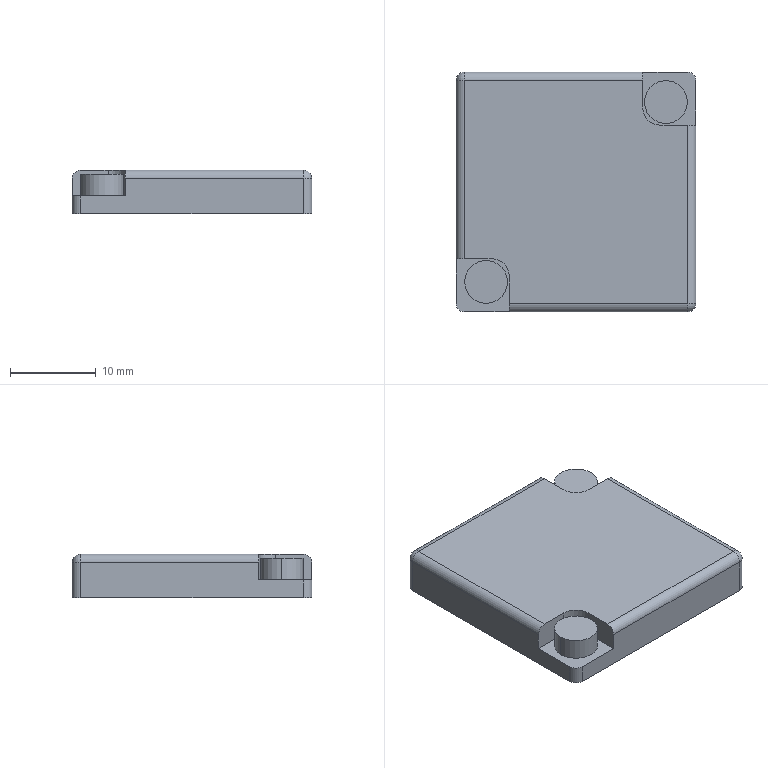Part | STEP file | AW30-03E_AW3020A Gauge_30 | 1 solid | 30 faces | box 28 x 28 x 5.1 mm | volume 3850 mm3 | cylinder 14 | plane 14 | sphere 2 | commonest cylinder face diameters 2 x8 5 x4 4 x2
STEP:
#1=CARTESIAN_POINT('',(-8.,-10.5,-0.5));
#2=VERTEX_POINT('',#1);
#3=CARTESIAN_POINT('',(-13.,-10.5,-0.5));
#4=VERTEX_POINT('',#3);
#5=CARTESIAN_POINT('',(-10.5,-10.5,-0.5));
#6=DIRECTION('',(0.,0.,1.));
#7=DIRECTION('',(-1.,0.,0.));
#8=AXIS2_PLACEMENT_3D('',#5,#6,#7);
#9=CIRCLE('',#8,2.5);
#10=EDGE_CURVE('',#2,#4,#9,.T.);
#11=ORIENTED_EDGE('',*,*,#10,.F.);
#12=CARTESIAN_POINT('',(-8.,-10.5,-3.));
#13=VERTEX_POINT('',#12);
#14=CARTESIAN_POINT('',(-8.,-10.5,-0.5));
#15=DIRECTION('',(0.,0.,-1.));
#16=VECTOR('',#15,1000.);
#17=LINE('',#14,#16);
#18=EDGE_CURVE('',#2,#13,#17,.T.);
#19=ORIENTED_EDGE('',*,*,#18,.T.);
#20=CARTESIAN_POINT('',(-13.,-10.5,-3.));
#21=VERTEX_POINT('',#20);
#22=CARTESIAN_POINT('',(-10.5,-10.5,-3.));
#23=DIRECTION('',(0.,0.,1.));
#24=DIRECTION('',(-1.,0.,0.));
#25=AXIS2_PLACEMENT_3D('',#22,#23,#24);
#26=CIRCLE('',#25,2.5);
#27=EDGE_CURVE('',#13,#21,#26,.T.);
#28=ORIENTED_EDGE('',*,*,#27,.T.);
#29=CARTESIAN_POINT('',(-13.,-10.5,-0.5));
#30=DIRECTION('',(0.,0.,-1.));
#31=VECTOR('',#30,1000.);
#32=LINE('',#29,#31);
#33=EDGE_CURVE('',#4,#21,#32,.T.);
#34=ORIENTED_EDGE('',*,*,#33,.F.);
#35=EDGE_LOOP('',(#11,#19,#28,#34));
#36=FACE_OUTER_BOUND('',#35,.T.);
#37=CARTESIAN_POINT('',(-10.5,-10.5,-0.5));
#38=DIRECTION('',(0.,0.,-1.));
#39=DIRECTION('',(-1.,0.,0.));
#40=AXIS2_PLACEMENT_3D('',#37,#38,#39);
#41=CYLINDRICAL_SURFACE('',#40,2.5);
#42=ADVANCED_FACE('',(#36),#41,.T.);
#43=CARTESIAN_POINT('',(13.,10.5,-0.5));
#44=VERTEX_POINT('',#43);
#45=CARTESIAN_POINT('',(8.,10.5,-0.5));
#46=VERTEX_POINT('',#45);
#47=CARTESIAN_POINT('',(10.5,10.5,-0.5));
#48=DIRECTION('',(0.,0.,1.));
#49=DIRECTION('',(1.,0.,0.));
#50=AXIS2_PLACEMENT_3D('',#47,#48,#49);
#51=CIRCLE('',#50,2.5);
#52=EDGE_CURVE('',#44,#46,#51,.T.);
#53=ORIENTED_EDGE('',*,*,#52,.F.);
#54=CARTESIAN_POINT('',(13.,10.5,-3.));
#55=VERTEX_POINT('',#54);
#56=CARTESIAN_POINT('',(13.,10.5,-0.5));
#57=DIRECTION('',(0.,0.,-1.));
#58=VECTOR('',#57,1000.);
#59=LINE('',#56,#58);
#60=EDGE_CURVE('',#44,#55,#59,.T.);
#61=ORIENTED_EDGE('',*,*,#60,.T.);
#62=CARTESIAN_POINT('',(8.,10.5,-3.));
#63=VERTEX_POINT('',#62);
#64=CARTESIAN_POINT('',(10.5,10.5,-3.));
#65=DIRECTION('',(0.,0.,1.));
#66=DIRECTION('',(1.,0.,0.));
#67=AXIS2_PLACEMENT_3D('',#64,#65,#66);
#68=CIRCLE('',#67,2.5);
#69=EDGE_CURVE('',#55,#63,#68,.T.);
#70=ORIENTED_EDGE('',*,*,#69,.T.);
#71=CARTESIAN_POINT('',(8.,10.5,-0.5));
#72=DIRECTION('',(0.,0.,-1.));
#73=VECTOR('',#72,1000.);
#74=LINE('',#71,#73);
#75=EDGE_CURVE('',#46,#63,#74,.T.);
#76=ORIENTED_EDGE('',*,*,#75,.F.);
#77=EDGE_LOOP('',(#53,#61,#70,#76));
#78=FACE_OUTER_BOUND('',#77,.T.);
#79=CARTESIAN_POINT('',(10.5,10.5,-0.5));
#80=DIRECTION('',(0.,0.,-1.));
#81=DIRECTION('',(-1.,0.,0.));
#82=AXIS2_PLACEMENT_3D('',#79,#80,#81);
#83=CYLINDRICAL_SURFACE('',#82,2.5);
#84=ADVANCED_FACE('',(#78),#83,.T.);
#85=CARTESIAN_POINT('',(-13.,-14.,-3.));
#86=VERTEX_POINT('',#85);
#87=CARTESIAN_POINT('',(-7.8,-14.,-3.));
#88=VERTEX_POINT('',#87);
#89=CARTESIAN_POINT('',(-14.,-14.,-3.));
#90=DIRECTION('',(1.,0.,0.));
#91=VECTOR('',#90,1000.);
#92=LINE('',#89,#91);
#93=EDGE_CURVE('',#86,#88,#92,.T.);
#94=ORIENTED_EDGE('',*,*,#93,.T.);
#95=CARTESIAN_POINT('',(-7.8,-9.8,-3.));
#96=VERTEX_POINT('',#95);
#97=CARTESIAN_POINT('',(-7.8,-14.,-3.));
#98=DIRECTION('',(0.,1.,0.));
#99=VECTOR('',#98,1000.);
#100=LINE('',#97,#99);
#101=EDGE_CURVE('',#88,#96,#100,.T.);
#102=ORIENTED_EDGE('',*,*,#101,.T.);
#103=CARTESIAN_POINT('',(-9.8,-7.8,-3.));
#104=VERTEX_POINT('',#103);
#105=CARTESIAN_POINT('',(-9.8,-9.8,-3.));
#106=DIRECTION('',(0.,0.,1.));
#107=DIRECTION('',(-1.,0.,0.));
#108=AXIS2_PLACEMENT_3D('',#105,#106,#107);
#109=CIRCLE('',#108,2.);
#110=EDGE_CURVE('',#96,#104,#109,.T.);
#111=ORIENTED_EDGE('',*,*,#110,.T.);
#112=CARTESIAN_POINT('',(-14.,-7.8,-3.));
#113=VERTEX_POINT('',#112);
#114=CARTESIAN_POINT('',(-14.,-7.8,-3.));
#115=DIRECTION('',(-1.,0.,0.));
#116=VECTOR('',#115,1000.);
#117=LINE('',#114,#116);
#118=EDGE_CURVE('',#104,#113,#117,.T.);
#119=ORIENTED_EDGE('',*,*,#118,.T.);
#120=CARTESIAN_POINT('',(-14.,-13.,-3.));
#121=VERTEX_POINT('',#120);
#122=CARTESIAN_POINT('',(-14.,-14.,-3.));
#123=DIRECTION('',(0.,-1.,0.));
#124=VECTOR('',#123,1000.);
#125=LINE('',#122,#124);
#126=EDGE_CURVE('',#113,#121,#125,.T.);
#127=ORIENTED_EDGE('',*,*,#126,.T.);
#128=CARTESIAN_POINT('',(-13.,-13.,-3.));
#129=DIRECTION('',(0.,0.,-1.));
#130=DIRECTION('',(1.,0.,0.));
#131=AXIS2_PLACEMENT_3D('',#128,#129,#130);
#132=CIRCLE('',#131,1.);
#133=EDGE_CURVE('',#86,#121,#132,.T.);
#134=ORIENTED_EDGE('',*,*,#133,.F.);
#135=EDGE_LOOP('',(#94,#102,#111,#119,#127,#134));
#136=FACE_OUTER_BOUND('',#135,.T.);
#137=CARTESIAN_POINT('',(-10.5,-10.5,-3.));
#138=DIRECTION('',(0.,0.,1.));
#139=DIRECTION('',(-1.,0.,0.));
#140=AXIS2_PLACEMENT_3D('',#137,#138,#139);
#141=CIRCLE('',#140,2.5);
#142=EDGE_CURVE('',#21,#13,#141,.T.);
#143=ORIENTED_EDGE('',*,*,#142,.F.);
#144=ORIENTED_EDGE('',*,*,#27,.F.);
#145=EDGE_LOOP('',(#143,#144));
#146=FACE_BOUND('',#145,.T.);
#147=CARTESIAN_POINT('',(-9.8,-9.8,-3.));
#148=DIRECTION('',(0.,0.,1.));
#149=DIRECTION('',(-1.,0.,0.));
#150=AXIS2_PLACEMENT_3D('',#147,#148,#149);
#151=PLANE('',#150);
#152=ADVANCED_FACE('',(#136,#146),#151,.T.);
#153=CARTESIAN_POINT('',(-13.,-14.,-5.1));
#154=VERTEX_POINT('',#153);
#155=CARTESIAN_POINT('',(-13.,-14.,-5.1));
#156=DIRECTION('',(0.,0.,-1.));
#157=VECTOR('',#156,1000.);
#158=LINE('',#155,#157);
#159=EDGE_CURVE('',#86,#154,#158,.T.);
#160=ORIENTED_EDGE('',*,*,#159,.F.);
#161=ORIENTED_EDGE('',*,*,#133,.T.);
#162=CARTESIAN_POINT('',(-14.,-13.,-5.1));
#163=VERTEX_POINT('',#162);
#164=CARTESIAN_POINT('',(-14.,-13.,-5.1));
#165=DIRECTION('',(0.,0.,1.));
#166=VECTOR('',#165,1000.);
#167=LINE('',#164,#166);
#168=EDGE_CURVE('',#163,#121,#167,.T.);
#169=ORIENTED_EDGE('',*,*,#168,.F.);
#170=CARTESIAN_POINT('',(-13.,-13.,-5.1));
#171=DIRECTION('',(0.,0.,-1.));
#172=DIRECTION('',(-1.,0.,0.));
#173=AXIS2_PLACEMENT_3D('',#170,#171,#172);
#174=CIRCLE('',#173,1.);
#175=EDGE_CURVE('',#154,#163,#174,.T.);
#176=ORIENTED_EDGE('',*,*,#175,.F.);
#177=EDGE_LOOP('',(#160,#161,#169,#176));
#178=FACE_OUTER_BOUND('',#177,.T.);
#179=CARTESIAN_POINT('',(-13.,-13.,-5.1));
#180=DIRECTION('',(0.,0.,1.));
#181=DIRECTION('',(1.,0.,0.));
#182=AXIS2_PLACEMENT_3D('',#179,#180,#181);
#183=CYLINDRICAL_SURFACE('',#182,1.);
#184=ADVANCED_FACE('',(#178),#183,.T.);
#185=CARTESIAN_POINT('',(13.,14.,-3.));
#186=VERTEX_POINT('',#185);
#187=CARTESIAN_POINT('',(7.8,14.,-3.));
#188=VERTEX_POINT('',#187);
#189=CARTESIAN_POINT('',(14.,14.,-3.));
#190=DIRECTION('',(-1.,0.,0.));
#191=VECTOR('',#190,1000.);
#192=LINE('',#189,#191);
#193=EDGE_CURVE('',#186,#188,#192,.T.);
#194=ORIENTED_EDGE('',*,*,#193,.T.);
#195=CARTESIAN_POINT('',(7.8,9.8,-3.));
#196=VERTEX_POINT('',#195);
#197=CARTESIAN_POINT('',(7.8,14.,-3.));
#198=DIRECTION('',(0.,-1.,0.));
#199=VECTOR('',#198,1000.);
#200=LINE('',#197,#199);
#201=EDGE_CURVE('',#188,#196,#200,.T.);
#202=ORIENTED_EDGE('',*,*,#201,.T.);
#203=CARTESIAN_POINT('',(9.8,7.8,-3.));
#204=VERTEX_POINT('',#203);
#205=CARTESIAN_POINT('',(9.8,9.8,-3.));
#206=DIRECTION('',(0.,0.,1.));
#207=DIRECTION('',(1.,0.,0.));
#208=AXIS2_PLACEMENT_3D('',#205,#206,#207);
#209=CIRCLE('',#208,2.);
#210=EDGE_CURVE('',#196,#204,#209,.T.);
#211=ORIENTED_EDGE('',*,*,#210,.T.);
#212=CARTESIAN_POINT('',(14.,7.8,-3.));
#213=VERTEX_POINT('',#212);
#214=CARTESIAN_POINT('',(14.,7.8,-3.));
#215=DIRECTION('',(1.,0.,0.));
#216=VECTOR('',#215,1000.);
#217=LINE('',#214,#216);
#218=EDGE_CURVE('',#204,#213,#217,.T.);
#219=ORIENTED_EDGE('',*,*,#218,.T.);
#220=CARTESIAN_POINT('',(14.,13.,-3.));
#221=VERTEX_POINT('',#220);
#222=CARTESIAN_POINT('',(14.,14.,-3.));
#223=DIRECTION('',(0.,1.,0.));
#224=VECTOR('',#223,1000.);
#225=LINE('',#222,#224);
#226=EDGE_CURVE('',#213,#221,#225,.T.);
#227=ORIENTED_EDGE('',*,*,#226,.T.);
#228=CARTESIAN_POINT('',(13.,13.,-3.));
#229=DIRECTION('',(0.,0.,-1.));
#230=DIRECTION('',(1.,0.,0.));
#231=AXIS2_PLACEMENT_3D('',#228,#229,#230);
#232=CIRCLE('',#231,1.);
#233=EDGE_CURVE('',#186,#221,#232,.T.);
#234=ORIENTED_EDGE('',*,*,#233,.F.);
#235=EDGE_LOOP('',(#194,#202,#211,#219,#227,#234));
#236=FACE_OUTER_BOUND('',#235,.T.);
#237=CARTESIAN_POINT('',(10.5,10.5,-3.));
#238=DIRECTION('',(0.,0.,1.));
#239=DIRECTION('',(1.,0.,0.));
#240=AXIS2_PLACEMENT_3D('',#237,#238,#239);
#241=CIRCLE('',#240,2.5);
#242=EDGE_CURVE('',#63,#55,#241,.T.);
#243=ORIENTED_EDGE('',*,*,#242,.F.);
#244=ORIENTED_EDGE('',*,*,#69,.F.);
#245=EDGE_LOOP('',(#243,#244));
#246=FACE_BOUND('',#245,.T.);
#247=CARTESIAN_POINT('',(9.8,9.8,-3.));
#248=DIRECTION('',(0.,0.,1.));
#249=DIRECTION('',(1.,0.,0.));
#250=AXIS2_PLACEMENT_3D('',#247,#248,#249);
#251=PLANE('',#250);
#252=ADVANCED_FACE('',(#236,#246),#251,.T.);
#253=CARTESIAN_POINT('',(13.,14.,-5.1));
#254=VERTEX_POINT('',#253);
#255=CARTESIAN_POINT('',(13.,14.,-5.1));
#256=DIRECTION('',(0.,0.,-1.));
#257=VECTOR('',#256,1000.);
#258=LINE('',#255,#257);
#259=EDGE_CURVE('',#186,#254,#258,.T.);
#260=ORIENTED_EDGE('',*,*,#259,.F.);
#261=ORIENTED_EDGE('',*,*,#233,.T.);
#262=CARTESIAN_POINT('',(14.,13.,-5.1));
#263=VERTEX_POINT('',#262);
#264=CARTESIAN_POINT('',(14.,13.,-5.1));
#265=DIRECTION('',(0.,0.,1.));
#266=VECTOR('',#265,1000.);
#267=LINE('',#264,#266);
#268=EDGE_CURVE('',#263,#221,#267,.T.);
#269=ORIENTED_EDGE('',*,*,#268,.F.);
#270=CARTESIAN_POINT('',(13.,13.,-5.1));
#271=DIRECTION('',(0.,0.,-1.));
#272=DIRECTION('',(-1.,0.,0.));
#273=AXIS2_PLACEMENT_3D('',#270,#271,#272);
#274=CIRCLE('',#273,1.);
#275=EDGE_CURVE('',#254,#263,#274,.T.);
#276=ORIENTED_EDGE('',*,*,#275,.F.);
#277=EDGE_LOOP('',(#260,#261,#269,#276));
#278=FACE_OUTER_BOUND('',#277,.T.);
#279=CARTESIAN_POINT('',(13.,13.,-5.1));
#280=DIRECTION('',(0.,0.,1.));
#281=DIRECTION('',(1.,0.,0.));
#282=AXIS2_PLACEMENT_3D('',#279,#280,#281);
#283=CYLINDRICAL_SURFACE('',#282,1.);
#284=ADVANCED_FACE('',(#278),#283,.T.);
#285=CARTESIAN_POINT('',(14.,7.8,-1.));
#286=VERTEX_POINT('',#285);
#287=CARTESIAN_POINT('',(14.,7.8,-3.));
#288=DIRECTION('',(0.,0.,1.));
#289=VECTOR('',#288,1000.);
#290=LINE('',#287,#289);
#291=EDGE_CURVE('',#213,#286,#290,.T.);
#292=ORIENTED_EDGE('',*,*,#291,.T.);
#293=CARTESIAN_POINT('',(14.,-13.,-1.));
#294=VERTEX_POINT('',#293);
#295=CARTESIAN_POINT('',(14.,-14.,-1.));
#296=DIRECTION('',(0.,-1.,0.));
#297=VECTOR('',#296,1000.);
#298=LINE('',#295,#297);
#299=EDGE_CURVE('',#286,#294,#298,.T.);
#300=ORIENTED_EDGE('',*,*,#299,.T.);
#301=CARTESIAN_POINT('',(14.,-13.,-5.1));
#302=VERTEX_POINT('',#301);
#303=CARTESIAN_POINT('',(14.,-13.,-5.1));
#304=DIRECTION('',(0.,0.,-1.));
#305=VECTOR('',#304,1000.);
#306=LINE('',#303,#305);
#307=EDGE_CURVE('',#294,#302,#306,.T.);
#308=ORIENTED_EDGE('',*,*,#307,.T.);
#309=CARTESIAN_POINT('',(14.,14.,-5.1));
#310=DIRECTION('',(0.,1.,0.));
#311=VECTOR('',#310,1000.);
#312=LINE('',#309,#311);
#313=EDGE_CURVE('',#302,#263,#312,.T.);
#314=ORIENTED_EDGE('',*,*,#313,.T.);
#315=ORIENTED_EDGE('',*,*,#268,.T.);
#316=ORIENTED_EDGE('',*,*,#226,.F.);
#317=EDGE_LOOP('',(#292,#300,#308,#314,#315,#316));
#318=FACE_OUTER_BOUND('',#317,.T.);
#319=CARTESIAN_POINT('',(14.,14.,-5.1));
#320=DIRECTION('',(1.,0.,0.));
#321=DIRECTION('',(0.,1.,0.));
#322=AXIS2_PLACEMENT_3D('',#319,#320,#321);
#323=PLANE('',#322);
#324=ADVANCED_FACE('',(#318),#323,.T.);
#325=CARTESIAN_POINT('',(-7.8,-14.,-1.));
#326=VERTEX_POINT('',#325);
#327=CARTESIAN_POINT('',(-7.8,-14.,-3.));
#328=DIRECTION('',(0.,0.,1.));
#329=VECTOR('',#328,1000.);
#330=LINE('',#327,#329);
#331=EDGE_CURVE('',#88,#326,#330,.T.);
#332=ORIENTED_EDGE('',*,*,#331,.F.);
#333=ORIENTED_EDGE('',*,*,#93,.F.);
#334=ORIENTED_EDGE('',*,*,#159,.T.);
#335=CARTESIAN_POINT('',(13.,-14.,-5.1));
#336=VERTEX_POINT('',#335);
#337=CARTESIAN_POINT('',(14.,-14.,-5.1));
#338=DIRECTION('',(1.,0.,0.));
#339=VECTOR('',#338,1000.);
#340=LINE('',#337,#339);
#341=EDGE_CURVE('',#154,#336,#340,.T.);
#342=ORIENTED_EDGE('',*,*,#341,.T.);
#343=CARTESIAN_POINT('',(13.,-14.,-1.));
#344=VERTEX_POINT('',#343);
#345=CARTESIAN_POINT('',(13.,-14.,-5.1));
#346=DIRECTION('',(0.,0.,1.));
#347=VECTOR('',#346,1000.);
#348=LINE('',#345,#347);
#349=EDGE_CURVE('',#336,#344,#348,.T.);
#350=ORIENTED_EDGE('',*,*,#349,.T.);
#351=CARTESIAN_POINT('',(-14.,-14.,-1.));
#352=DIRECTION('',(-1.,0.,0.));
#353=VECTOR('',#352,1000.);
#354=LINE('',#351,#353);
#355=EDGE_CURVE('',#344,#326,#354,.T.);
#356=ORIENTED_EDGE('',*,*,#355,.T.);
#357=EDGE_LOOP('',(#332,#333,#334,#342,#350,#356));
#358=FACE_OUTER_BOUND('',#357,.T.);
#359=CARTESIAN_POINT('',(14.,-14.,-5.1));
#360=DIRECTION('',(0.,-1.,0.));
#361=DIRECTION('',(1.,0.,0.));
#362=AXIS2_PLACEMENT_3D('',#359,#360,#361);
#363=PLANE('',#362);
#364=ADVANCED_FACE('',(#358),#363,.T.);
#365=CARTESIAN_POINT('',(-14.,-7.8,-1.));
#366=VERTEX_POINT('',#365);
#367=CARTESIAN_POINT('',(-14.,-7.8,-3.));
#368=DIRECTION('',(0.,0.,1.));
#369=VECTOR('',#368,1000.);
#370=LINE('',#367,#369);
#371=EDGE_CURVE('',#113,#366,#370,.T.);
#372=ORIENTED_EDGE('',*,*,#371,.T.);
#373=CARTESIAN_POINT('',(-14.,13.,-1.));
#374=VERTEX_POINT('',#373);
#375=CARTESIAN_POINT('',(-14.,14.,-1.));
#376=DIRECTION('',(0.,1.,0.));
#377=VECTOR('',#376,1000.);
#378=LINE('',#375,#377);
#379=EDGE_CURVE('',#366,#374,#378,.T.);
#380=ORIENTED_EDGE('',*,*,#379,.T.);
#381=CARTESIAN_POINT('',(-14.,13.,-5.1));
#382=VERTEX_POINT('',#381);
#383=CARTESIAN_POINT('',(-14.,13.,-5.1));
#384=DIRECTION('',(0.,0.,-1.));
#385=VECTOR('',#384,1000.);
#386=LINE('',#383,#385);
#387=EDGE_CURVE('',#374,#382,#386,.T.);
#388=ORIENTED_EDGE('',*,*,#387,.T.);
#389=CARTESIAN_POINT('',(-14.,14.,-5.1));
#390=DIRECTION('',(0.,-1.,0.));
#391=VECTOR('',#390,1000.);
#392=LINE('',#389,#391);
#393=EDGE_CURVE('',#382,#163,#392,.T.);
#394=ORIENTED_EDGE('',*,*,#393,.T.);
#395=ORIENTED_EDGE('',*,*,#168,.T.);
#396=ORIENTED_EDGE('',*,*,#126,.F.);
#397=EDGE_LOOP('',(#372,#380,#388,#394,#395,#396));
#398=FACE_OUTER_BOUND('',#397,.T.);
#399=CARTESIAN_POINT('',(-14.,14.,-5.1));
#400=DIRECTION('',(-1.,0.,0.));
#401=DIRECTION('',(0.,-1.,0.));
#402=AXIS2_PLACEMENT_3D('',#399,#400,#401);
#403=PLANE('',#402);
#404=ADVANCED_FACE('',(#398),#403,.T.);
#405=CARTESIAN_POINT('',(7.8,14.,-1.));
#406=VERTEX_POINT('',#405);
#407=CARTESIAN_POINT('',(7.8,14.,-3.));
#408=DIRECTION('',(0.,0.,1.));
#409=VECTOR('',#408,1000.);
#410=LINE('',#407,#409);
#411=EDGE_CURVE('',#188,#406,#410,.T.);
#412=ORIENTED_EDGE('',*,*,#411,.F.);
#413=ORIENTED_EDGE('',*,*,#193,.F.);
#414=ORIENTED_EDGE('',*,*,#259,.T.);
#415=CARTESIAN_POINT('',(-13.,14.,-5.1));
#416=VERTEX_POINT('',#415);
#417=CARTESIAN_POINT('',(14.,14.,-5.1));
#418=DIRECTION('',(-1.,0.,0.));
#419=VECTOR('',#418,1000.);
#420=LINE('',#417,#419);
#421=EDGE_CURVE('',#254,#416,#420,.T.);
#422=ORIENTED_EDGE('',*,*,#421,.T.);
#423=CARTESIAN_POINT('',(-13.,14.,-1.));
#424=VERTEX_POINT('',#423);
#425=CARTESIAN_POINT('',(-13.,14.,-5.1));
#426=DIRECTION('',(0.,0.,1.));
#427=VECTOR('',#426,1000.);
#428=LINE('',#425,#427);
#429=EDGE_CURVE('',#416,#424,#428,.T.);
#430=ORIENTED_EDGE('',*,*,#429,.T.);
#431=CARTESIAN_POINT('',(14.,14.,-1.));
#432=DIRECTION('',(1.,0.,0.));
#433=VECTOR('',#432,1000.);
#434=LINE('',#431,#433);
#435=EDGE_CURVE('',#424,#406,#434,.T.);
#436=ORIENTED_EDGE('',*,*,#435,.T.);
#437=EDGE_LOOP('',(#412,#413,#414,#422,#430,#436));
#438=FACE_OUTER_BOUND('',#437,.T.);
#439=CARTESIAN_POINT('',(14.,14.,-5.1));
#440=DIRECTION('',(0.,1.,0.));
#441=DIRECTION('',(-1.,0.,0.));
#442=AXIS2_PLACEMENT_3D('',#439,#440,#441);
#443=PLANE('',#442);
#444=ADVANCED_FACE('',(#438),#443,.T.);
#445=ORIENTED_EDGE('',*,*,#421,.F.);
#446=ORIENTED_EDGE('',*,*,#275,.T.);
#447=ORIENTED_EDGE('',*,*,#313,.F.);
#448=CARTESIAN_POINT('',(13.,-13.,-5.1));
#449=DIRECTION('',(0.,0.,-1.));
#450=DIRECTION('',(-1.,0.,0.));
#451=AXIS2_PLACEMENT_3D('',#448,#449,#450);
#452=CIRCLE('',#451,1.);
#453=EDGE_CURVE('',#302,#336,#452,.T.);
#454=ORIENTED_EDGE('',*,*,#453,.T.);
#455=ORIENTED_EDGE('',*,*,#341,.F.);
#456=ORIENTED_EDGE('',*,*,#175,.T.);
#457=ORIENTED_EDGE('',*,*,#393,.F.);
#458=CARTESIAN_POINT('',(-13.,13.,-5.1));
#459=DIRECTION('',(0.,0.,-1.));
#460=DIRECTION('',(-1.,0.,0.));
#461=AXIS2_PLACEMENT_3D('',#458,#459,#460);
#462=CIRCLE('',#461,1.);
#463=EDGE_CURVE('',#382,#416,#462,.T.);
#464=ORIENTED_EDGE('',*,*,#463,.T.);
#465=EDGE_LOOP('',(#445,#446,#447,#454,#455,#456,#457,#464));
#466=FACE_OUTER_BOUND('',#465,.T.);
#467=CARTESIAN_POINT('',(14.,-14.,-5.1));
#468=DIRECTION('',(0.,0.,-1.));
#469=DIRECTION('',(-1.,0.,0.));
#470=AXIS2_PLACEMENT_3D('',#467,#468,#469);
#471=PLANE('',#470);
#472=ADVANCED_FACE('',(#466),#471,.T.);
#473=CARTESIAN_POINT('',(-13.,13.,0.));
#474=VERTEX_POINT('',#473);
#475=CARTESIAN_POINT('',(-13.,-7.8,0.));
#476=VERTEX_POINT('',#475);
#477=CARTESIAN_POINT('',(-13.,-14.,0.));
#478=DIRECTION('',(0.,-1.,0.));
#479=VECTOR('',#478,1000.);
#480=LINE('',#477,#479);
#481=EDGE_CURVE('',#474,#476,#480,.T.);
#482=ORIENTED_EDGE('',*,*,#481,.T.);
#483=CARTESIAN_POINT('',(-9.8,-7.8,0.));
#484=VERTEX_POINT('',#483);
#485=CARTESIAN_POINT('',(-14.,-7.8,0.));
#486=DIRECTION('',(-1.,0.,0.));
#487=VECTOR('',#486,1000.);
#488=LINE('',#485,#487);
#489=EDGE_CURVE('',#484,#476,#488,.T.);
#490=ORIENTED_EDGE('',*,*,#489,.F.);
#491=CARTESIAN_POINT('',(-7.8,-9.8,0.));
#492=VERTEX_POINT('',#491);
#493=CARTESIAN_POINT('',(-9.8,-9.8,0.));
#494=DIRECTION('',(0.,0.,1.));
#495=DIRECTION('',(-1.,0.,0.));
#496=AXIS2_PLACEMENT_3D('',#493,#494,#495);
#497=CIRCLE('',#496,2.);
#498=EDGE_CURVE('',#492,#484,#497,.T.);
#499=ORIENTED_EDGE('',*,*,#498,.F.);
#500=CARTESIAN_POINT('',(-7.8,-13.,0.));
#501=VERTEX_POINT('',#500);
#502=CARTESIAN_POINT('',(-7.8,-14.,0.));
#503=DIRECTION('',(0.,1.,0.));
#504=VECTOR('',#503,1000.);
#505=LINE('',#502,#504);
#506=EDGE_CURVE('',#501,#492,#505,.T.);
#507=ORIENTED_EDGE('',*,*,#506,.F.);
#508=CARTESIAN_POINT('',(13.,-13.,0.));
#509=VERTEX_POINT('',#508);
#510=CARTESIAN_POINT('',(14.,-13.,0.));
#511=DIRECTION('',(1.,0.,0.));
#512=VECTOR('',#511,1000.);
#513=LINE('',#510,#512);
#514=EDGE_CURVE('',#501,#509,#513,.T.);
#515=ORIENTED_EDGE('',*,*,#514,.T.);
#516=CARTESIAN_POINT('',(13.,7.8,0.));
#517=VERTEX_POINT('',#516);
#518=CARTESIAN_POINT('',(13.,14.,0.));
#519=DIRECTION('',(0.,1.,0.));
#520=VECTOR('',#519,1000.);
#521=LINE('',#518,#520);
#522=EDGE_CURVE('',#509,#517,#521,.T.);
#523=ORIENTED_EDGE('',*,*,#522,.T.);
#524=CARTESIAN_POINT('',(9.8,7.8,0.));
#525=VERTEX_POINT('',#524);
#526=CARTESIAN_POINT('',(14.,7.8,0.));
#527=DIRECTION('',(1.,0.,0.));
#528=VECTOR('',#527,1000.);
#529=LINE('',#526,#528);
#530=EDGE_CURVE('',#525,#517,#529,.T.);
#531=ORIENTED_EDGE('',*,*,#530,.F.);
#532=CARTESIAN_POINT('',(7.8,9.8,0.));
#533=VERTEX_POINT('',#532);
#534=CARTESIAN_POINT('',(9.8,9.8,0.));
#535=DIRECTION('',(0.,0.,1.));
#536=DIRECTION('',(1.,0.,0.));
#537=AXIS2_PLACEMENT_3D('',#534,#535,#536);
#538=CIRCLE('',#537,2.);
#539=EDGE_CURVE('',#533,#525,#538,.T.);
#540=ORIENTED_EDGE('',*,*,#539,.F.);
#541=CARTESIAN_POINT('',(7.8,13.,0.));
#542=VERTEX_POINT('',#541);
#543=CARTESIAN_POINT('',(7.8,14.,0.));
#544=DIRECTION('',(0.,-1.,0.));
#545=VECTOR('',#544,1000.);
#546=LINE('',#543,#545);
#547=EDGE_CURVE('',#542,#533,#546,.T.);
#548=ORIENTED_EDGE('',*,*,#547,.F.);
#549=CARTESIAN_POINT('',(-14.,13.,0.));
#550=DIRECTION('',(-1.,0.,0.));
#551=VECTOR('',#550,1000.);
#552=LINE('',#549,#551);
#553=EDGE_CURVE('',#542,#474,#552,.T.);
#554=ORIENTED_EDGE('',*,*,#553,.T.);
#555=EDGE_LOOP('',(#482,#490,#499,#507,#515,#523,#531,#540,#548,#554));
#556=FACE_OUTER_BOUND('',#555,.T.);
#557=CARTESIAN_POINT('',(14.,-14.,0.));
#558=DIRECTION('',(0.,0.,-1.));
#559=DIRECTION('',(-1.,0.,0.));
#560=AXIS2_PLACEMENT_3D('',#557,#558,#559);
#561=PLANE('',#560);
#562=ADVANCED_FACE('',(#556),#561,.F.);
#563=ORIENTED_EDGE('',*,*,#453,.F.);
#564=ORIENTED_EDGE('',*,*,#307,.F.);
#565=CARTESIAN_POINT('',(13.,-13.,-1.));
#566=DIRECTION('',(0.,0.,1.));
#567=DIRECTION('',(1.,0.,0.));
#568=AXIS2_PLACEMENT_3D('',#565,#566,#567);
#569=CIRCLE('',#568,1.);
#570=EDGE_CURVE('',#344,#294,#569,.T.);
#571=ORIENTED_EDGE('',*,*,#570,.F.);
#572=ORIENTED_EDGE('',*,*,#349,.F.);
#573=EDGE_LOOP('',(#563,#564,#571,#572));
#574=FACE_OUTER_BOUND('',#573,.T.);
#575=CARTESIAN_POINT('',(13.,-13.,-5.1));
#576=DIRECTION('',(0.,0.,1.));
#577=DIRECTION('',(1.,0.,0.));
#578=AXIS2_PLACEMENT_3D('',#575,#576,#577);
#579=CYLINDRICAL_SURFACE('',#578,1.);
#580=ADVANCED_FACE('',(#574),#579,.T.);
#581=CARTESIAN_POINT('',(-7.8,-13.,-1.));
#582=DIRECTION('',(-1.,0.,0.));
#583=DIRECTION('',(0.,1.,0.));
#584=AXIS2_PLACEMENT_3D('',#581,#582,#583);
#585=CIRCLE('',#584,1.);
#586=EDGE_CURVE('',#326,#501,#585,.T.);
#587=ORIENTED_EDGE('',*,*,#586,.F.);
#588=ORIENTED_EDGE('',*,*,#355,.F.);
#589=CARTESIAN_POINT('',(13.,-13.,-1.));
#590=DIRECTION('',(1.,0.,0.));
#591=DIRECTION('',(0.,0.,-1.));
#592=AXIS2_PLACEMENT_3D('',#589,#590,#591);
#593=CIRCLE('',#592,1.);
#594=EDGE_CURVE('',#509,#344,#593,.T.);
#595=ORIENTED_EDGE('',*,*,#594,.F.);
#596=ORIENTED_EDGE('',*,*,#514,.F.);
#597=EDGE_LOOP('',(#587,#588,#595,#596));
#598=FACE_OUTER_BOUND('',#597,.T.);
#599=CARTESIAN_POINT('',(14.,-13.,-1.));
#600=DIRECTION('',(-1.,0.,0.));
#601=DIRECTION('',(0.,-1.,0.));
#602=AXIS2_PLACEMENT_3D('',#599,#600,#601);
#603=CYLINDRICAL_SURFACE('',#602,1.);
#604=ADVANCED_FACE('',(#598),#603,.T.);
#605=ORIENTED_EDGE('',*,*,#594,.T.);
#606=ORIENTED_EDGE('',*,*,#570,.T.);
#607=CARTESIAN_POINT('',(13.,-13.,-1.));
#608=DIRECTION('',(0.,1.,0.));
#609=DIRECTION('',(0.,0.,-1.));
#610=AXIS2_PLACEMENT_3D('',#607,#608,#609);
#611=CIRCLE('',#610,1.);
#612=EDGE_CURVE('',#509,#294,#611,.T.);
#613=ORIENTED_EDGE('',*,*,#612,.F.);
#614=EDGE_LOOP('',(#605,#606,#613));
#615=FACE_OUTER_BOUND('',#614,.T.);
#616=CARTESIAN_POINT('',(13.,-13.,-1.));
#617=DIRECTION('',(0.,1.,0.));
#618=DIRECTION('',(1.,0.,0.));
#619=AXIS2_PLACEMENT_3D('',#616,#617,#618);
#620=SPHERICAL_SURFACE('',#619,1.);
#621=ADVANCED_FACE('',(#615),#620,.T.);
#622=CARTESIAN_POINT('',(13.,7.8,-1.));
#623=DIRECTION('',(0.,1.,0.));
#624=DIRECTION('',(1.,0.,0.));
#625=AXIS2_PLACEMENT_3D('',#622,#623,#624);
#626=CIRCLE('',#625,1.);
#627=EDGE_CURVE('',#517,#286,#626,.T.);
#628=ORIENTED_EDGE('',*,*,#627,.F.);
#629=ORIENTED_EDGE('',*,*,#522,.F.);
#630=ORIENTED_EDGE('',*,*,#612,.T.);
#631=ORIENTED_EDGE('',*,*,#299,.F.);
#632=EDGE_LOOP('',(#628,#629,#630,#631));
#633=FACE_OUTER_BOUND('',#632,.T.);
#634=CARTESIAN_POINT('',(13.,-14.,-1.));
#635=DIRECTION('',(0.,-1.,0.));
#636=DIRECTION('',(1.,0.,0.));
#637=AXIS2_PLACEMENT_3D('',#634,#635,#636);
#638=CYLINDRICAL_SURFACE('',#637,1.);
#639=ADVANCED_FACE('',(#633),#638,.T.);
#640=CARTESIAN_POINT('',(-13.,-7.8,-1.));
#641=DIRECTION('',(0.,-1.,0.));
#642=DIRECTION('',(-1.,0.,0.));
#643=AXIS2_PLACEMENT_3D('',#640,#641,#642);
#644=CIRCLE('',#643,1.);
#645=EDGE_CURVE('',#476,#366,#644,.T.);
#646=ORIENTED_EDGE('',*,*,#645,.F.);
#647=ORIENTED_EDGE('',*,*,#481,.F.);
#648=CARTESIAN_POINT('',(-13.,13.,-1.));
#649=DIRECTION('',(0.,1.,0.));
#650=DIRECTION('',(0.,0.,1.));
#651=AXIS2_PLACEMENT_3D('',#648,#649,#650);
#652=CIRCLE('',#651,1.);
#653=EDGE_CURVE('',#374,#474,#652,.T.);
#654=ORIENTED_EDGE('',*,*,#653,.F.);
#655=ORIENTED_EDGE('',*,*,#379,.F.);
#656=EDGE_LOOP('',(#646,#647,#654,#655));
#657=FACE_OUTER_BOUND('',#656,.T.);
#658=CARTESIAN_POINT('',(-13.,-14.,-1.));
#659=DIRECTION('',(0.,1.,0.));
#660=DIRECTION('',(-1.,0.,0.));
#661=AXIS2_PLACEMENT_3D('',#658,#659,#660);
#662=CYLINDRICAL_SURFACE('',#661,1.);
#663=ADVANCED_FACE('',(#657),#662,.T.);
#664=ORIENTED_EDGE('',*,*,#463,.F.);
#665=ORIENTED_EDGE('',*,*,#387,.F.);
#666=CARTESIAN_POINT('',(-13.,13.,-1.));
#667=DIRECTION('',(0.,0.,1.));
#668=DIRECTION('',(1.,0.,0.));
#669=AXIS2_PLACEMENT_3D('',#666,#667,#668);
#670=CIRCLE('',#669,1.);
#671=EDGE_CURVE('',#424,#374,#670,.T.);
#672=ORIENTED_EDGE('',*,*,#671,.F.);
#673=ORIENTED_EDGE('',*,*,#429,.F.);
#674=EDGE_LOOP('',(#664,#665,#672,#673));
#675=FACE_OUTER_BOUND('',#674,.T.);
#676=CARTESIAN_POINT('',(-13.,13.,-5.1));
#677=DIRECTION('',(0.,0.,1.));
#678=DIRECTION('',(1.,0.,0.));
#679=AXIS2_PLACEMENT_3D('',#676,#677,#678);
#680=CYLINDRICAL_SURFACE('',#679,1.);
#681=ADVANCED_FACE('',(#675),#680,.T.);
#682=ORIENTED_EDGE('',*,*,#671,.T.);
#683=ORIENTED_EDGE('',*,*,#653,.T.);
#684=CARTESIAN_POINT('',(-13.,13.,-1.));
#685=DIRECTION('',(1.,0.,0.));
#686=DIRECTION('',(0.,-1.,0.));
#687=AXIS2_PLACEMENT_3D('',#684,#685,#686);
#688=CIRCLE('',#687,1.);
#689=EDGE_CURVE('',#424,#474,#688,.T.);
#690=ORIENTED_EDGE('',*,*,#689,.F.);
#691=EDGE_LOOP('',(#682,#683,#690));
#692=FACE_OUTER_BOUND('',#691,.T.);
#693=CARTESIAN_POINT('',(-13.,13.,-1.));
#694=DIRECTION('',(0.,1.,0.));
#695=DIRECTION('',(1.,0.,0.));
#696=AXIS2_PLACEMENT_3D('',#693,#694,#695);
#697=SPHERICAL_SURFACE('',#696,1.);
#698=ADVANCED_FACE('',(#692),#697,.T.);
#699=CARTESIAN_POINT('',(7.8,13.,-1.));
#700=DIRECTION('',(1.,0.,0.));
#701=DIRECTION('',(0.,-1.,0.));
#702=AXIS2_PLACEMENT_3D('',#699,#700,#701);
#703=CIRCLE('',#702,1.);
#704=EDGE_CURVE('',#406,#542,#703,.T.);
#705=ORIENTED_EDGE('',*,*,#704,.F.);
#706=ORIENTED_EDGE('',*,*,#435,.F.);
#707=ORIENTED_EDGE('',*,*,#689,.T.);
#708=ORIENTED_EDGE('',*,*,#553,.F.);
#709=EDGE_LOOP('',(#705,#706,#707,#708));
#710=FACE_OUTER_BOUND('',#709,.T.);
#711=CARTESIAN_POINT('',(14.,13.,-1.));
#712=DIRECTION('',(1.,0.,0.));
#713=DIRECTION('',(0.,1.,0.));
#714=AXIS2_PLACEMENT_3D('',#711,#712,#713);
#715=CYLINDRICAL_SURFACE('',#714,1.);
#716=ADVANCED_FACE('',(#710),#715,.T.);
#717=ORIENTED_EDGE('',*,*,#627,.T.);
#718=ORIENTED_EDGE('',*,*,#291,.F.);
#719=ORIENTED_EDGE('',*,*,#218,.F.);
#720=CARTESIAN_POINT('',(9.8,7.8,-3.));
#721=DIRECTION('',(0.,0.,1.));
#722=VECTOR('',#721,1000.);
#723=LINE('',#720,#722);
#724=EDGE_CURVE('',#204,#525,#723,.T.);
#725=ORIENTED_EDGE('',*,*,#724,.T.);
#726=ORIENTED_EDGE('',*,*,#530,.T.);
#727=EDGE_LOOP('',(#717,#718,#719,#725,#726));
#728=FACE_OUTER_BOUND('',#727,.T.);
#729=CARTESIAN_POINT('',(14.,7.8,-3.));
#730=DIRECTION('',(0.,-1.,0.));
#731=DIRECTION('',(1.,0.,0.));
#732=AXIS2_PLACEMENT_3D('',#729,#730,#731);
#733=PLANE('',#732);
#734=ADVANCED_FACE('',(#728),#733,.F.);
#735=ORIENTED_EDGE('',*,*,#539,.T.);
#736=ORIENTED_EDGE('',*,*,#724,.F.);
#737=ORIENTED_EDGE('',*,*,#210,.F.);
#738=CARTESIAN_POINT('',(7.8,9.8,-3.));
#739=DIRECTION('',(0.,0.,1.));
#740=VECTOR('',#739,1000.);
#741=LINE('',#738,#740);
#742=EDGE_CURVE('',#196,#533,#741,.T.);
#743=ORIENTED_EDGE('',*,*,#742,.T.);
#744=EDGE_LOOP('',(#735,#736,#737,#743));
#745=FACE_OUTER_BOUND('',#744,.T.);
#746=CARTESIAN_POINT('',(9.8,9.8,-3.));
#747=DIRECTION('',(0.,0.,1.));
#748=DIRECTION('',(1.,0.,0.));
#749=AXIS2_PLACEMENT_3D('',#746,#747,#748);
#750=CYLINDRICAL_SURFACE('',#749,2.);
#751=ADVANCED_FACE('',(#745),#750,.F.);
#752=ORIENTED_EDGE('',*,*,#704,.T.);
#753=ORIENTED_EDGE('',*,*,#547,.T.);
#754=ORIENTED_EDGE('',*,*,#742,.F.);
#755=ORIENTED_EDGE('',*,*,#201,.F.);
#756=ORIENTED_EDGE('',*,*,#411,.T.);
#757=EDGE_LOOP('',(#752,#753,#754,#755,#756));
#758=FACE_OUTER_BOUND('',#757,.T.);
#759=CARTESIAN_POINT('',(7.8,14.,-3.));
#760=DIRECTION('',(-1.,0.,0.));
#761=DIRECTION('',(0.,-1.,0.));
#762=AXIS2_PLACEMENT_3D('',#759,#760,#761);
#763=PLANE('',#762);
#764=ADVANCED_FACE('',(#758),#763,.F.);
#765=ORIENTED_EDGE('',*,*,#60,.F.);
#766=CARTESIAN_POINT('',(10.5,10.5,-0.5));
#767=DIRECTION('',(0.,0.,1.));
#768=DIRECTION('',(1.,0.,0.));
#769=AXIS2_PLACEMENT_3D('',#766,#767,#768);
#770=CIRCLE('',#769,2.5);
#771=EDGE_CURVE('',#46,#44,#770,.T.);
#772=ORIENTED_EDGE('',*,*,#771,.F.);
#773=ORIENTED_EDGE('',*,*,#75,.T.);
#774=ORIENTED_EDGE('',*,*,#242,.T.);
#775=EDGE_LOOP('',(#765,#772,#773,#774));
#776=FACE_OUTER_BOUND('',#775,.T.);
#777=CARTESIAN_POINT('',(10.5,10.5,-0.5));
#778=DIRECTION('',(0.,0.,-1.));
#779=DIRECTION('',(-1.,0.,0.));
#780=AXIS2_PLACEMENT_3D('',#777,#778,#779);
#781=CYLINDRICAL_SURFACE('',#780,2.5);
#782=ADVANCED_FACE('',(#776),#781,.T.);
#783=ORIENTED_EDGE('',*,*,#771,.T.);
#784=ORIENTED_EDGE('',*,*,#52,.T.);
#785=EDGE_LOOP('',(#783,#784));
#786=FACE_OUTER_BOUND('',#785,.T.);
#787=CARTESIAN_POINT('',(10.5,10.5,-0.5));
#788=DIRECTION('',(0.,0.,1.));
#789=DIRECTION('',(1.,0.,0.));
#790=AXIS2_PLACEMENT_3D('',#787,#788,#789);
#791=PLANE('',#790);
#792=ADVANCED_FACE('',(#786),#791,.T.);
#793=ORIENTED_EDGE('',*,*,#645,.T.);
#794=ORIENTED_EDGE('',*,*,#371,.F.);
#795=ORIENTED_EDGE('',*,*,#118,.F.);
#796=CARTESIAN_POINT('',(-9.8,-7.8,-3.));
#797=DIRECTION('',(0.,0.,1.));
#798=VECTOR('',#797,1000.);
#799=LINE('',#796,#798);
#800=EDGE_CURVE('',#104,#484,#799,.T.);
#801=ORIENTED_EDGE('',*,*,#800,.T.);
#802=ORIENTED_EDGE('',*,*,#489,.T.);
#803=EDGE_LOOP('',(#793,#794,#795,#801,#802));
#804=FACE_OUTER_BOUND('',#803,.T.);
#805=CARTESIAN_POINT('',(-14.,-7.8,-3.));
#806=DIRECTION('',(0.,1.,0.));
#807=DIRECTION('',(-1.,0.,0.));
#808=AXIS2_PLACEMENT_3D('',#805,#806,#807);
#809=PLANE('',#808);
#810=ADVANCED_FACE('',(#804),#809,.F.);
#811=ORIENTED_EDGE('',*,*,#498,.T.);
#812=ORIENTED_EDGE('',*,*,#800,.F.);
#813=ORIENTED_EDGE('',*,*,#110,.F.);
#814=CARTESIAN_POINT('',(-7.8,-9.8,-3.));
#815=DIRECTION('',(0.,0.,1.));
#816=VECTOR('',#815,1000.);
#817=LINE('',#814,#816);
#818=EDGE_CURVE('',#96,#492,#817,.T.);
#819=ORIENTED_EDGE('',*,*,#818,.T.);
#820=EDGE_LOOP('',(#811,#812,#813,#819));
#821=FACE_OUTER_BOUND('',#820,.T.);
#822=CARTESIAN_POINT('',(-9.8,-9.8,-3.));
#823=DIRECTION('',(0.,0.,1.));
#824=DIRECTION('',(1.,0.,0.));
#825=AXIS2_PLACEMENT_3D('',#822,#823,#824);
#826=CYLINDRICAL_SURFACE('',#825,2.);
#827=ADVANCED_FACE('',(#821),#826,.F.);
#828=ORIENTED_EDGE('',*,*,#586,.T.);
#829=ORIENTED_EDGE('',*,*,#506,.T.);
#830=ORIENTED_EDGE('',*,*,#818,.F.);
#831=ORIENTED_EDGE('',*,*,#101,.F.);
#832=ORIENTED_EDGE('',*,*,#331,.T.);
#833=EDGE_LOOP('',(#828,#829,#830,#831,#832));
#834=FACE_OUTER_BOUND('',#833,.T.);
#835=CARTESIAN_POINT('',(-7.8,-14.,-3.));
#836=DIRECTION('',(1.,0.,0.));
#837=DIRECTION('',(0.,1.,0.));
#838=AXIS2_PLACEMENT_3D('',#835,#836,#837);
#839=PLANE('',#838);
#840=ADVANCED_FACE('',(#834),#839,.F.);
#841=ORIENTED_EDGE('',*,*,#18,.F.);
#842=CARTESIAN_POINT('',(-10.5,-10.5,-0.5));
#843=DIRECTION('',(0.,0.,1.));
#844=DIRECTION('',(-1.,0.,0.));
#845=AXIS2_PLACEMENT_3D('',#842,#843,#844);
#846=CIRCLE('',#845,2.5);
#847=EDGE_CURVE('',#4,#2,#846,.T.);
#848=ORIENTED_EDGE('',*,*,#847,.F.);
#849=ORIENTED_EDGE('',*,*,#33,.T.);
#850=ORIENTED_EDGE('',*,*,#142,.T.);
#851=EDGE_LOOP('',(#841,#848,#849,#850));
#852=FACE_OUTER_BOUND('',#851,.T.);
#853=CARTESIAN_POINT('',(-10.5,-10.5,-0.5));
#854=DIRECTION('',(0.,0.,-1.));
#855=DIRECTION('',(-1.,0.,0.));
#856=AXIS2_PLACEMENT_3D('',#853,#854,#855);
#857=CYLINDRICAL_SURFACE('',#856,2.5);
#858=ADVANCED_FACE('',(#852),#857,.T.);
#859=ORIENTED_EDGE('',*,*,#847,.T.);
#860=ORIENTED_EDGE('',*,*,#10,.T.);
#861=EDGE_LOOP('',(#859,#860));
#862=FACE_OUTER_BOUND('',#861,.T.);
#863=CARTESIAN_POINT('',(-10.5,-10.5,-0.5));
#864=DIRECTION('',(0.,0.,1.));
#865=DIRECTION('',(-1.,0.,0.));
#866=AXIS2_PLACEMENT_3D('',#863,#864,#865);
#867=PLANE('',#866);
#868=ADVANCED_FACE('',(#862),#867,.T.);
#869=CLOSED_SHELL('',(#42,#84,#152,#184,#252,#284,#324,#364,#404,#444,#472,#562,#580,#604,#621,#639,#663,#681,#698,#716,#734,#751,#764,#782,#792,#810,#827,#840,#858,#868));
#870=MANIFOLD_SOLID_BREP('',#869);
#871=CARTESIAN_POINT('',(0.,0.,0.));
#872=DIRECTION('',(0.,0.,1.));
#873=DIRECTION('',(1.,0.,0.));
#874=AXIS2_PLACEMENT_3D('',#871,#872,#873);
#875=(LENGTH_UNIT()NAMED_UNIT(*)SI_UNIT(.MILLI.,.METRE.));
#876=UNCERTAINTY_MEASURE_WITH_UNIT(LENGTH_MEASURE(0.00001),#875,'','');
#877=(NAMED_UNIT(*)PLANE_ANGLE_UNIT()SI_UNIT($,.RADIAN.));
#878=(NAMED_UNIT(*)SI_UNIT($,.STERADIAN.)SOLID_ANGLE_UNIT());
#879=(GEOMETRIC_REPRESENTATION_CONTEXT(3)GLOBAL_UNCERTAINTY_ASSIGNED_CONTEXT((#876))GLOBAL_UNIT_ASSIGNED_CONTEXT((#875,#877,#878))REPRESENTATION_CONTEXT('',''));
#880=ADVANCED_BREP_SHAPE_REPRESENTATION('',(#870,#874),#879);